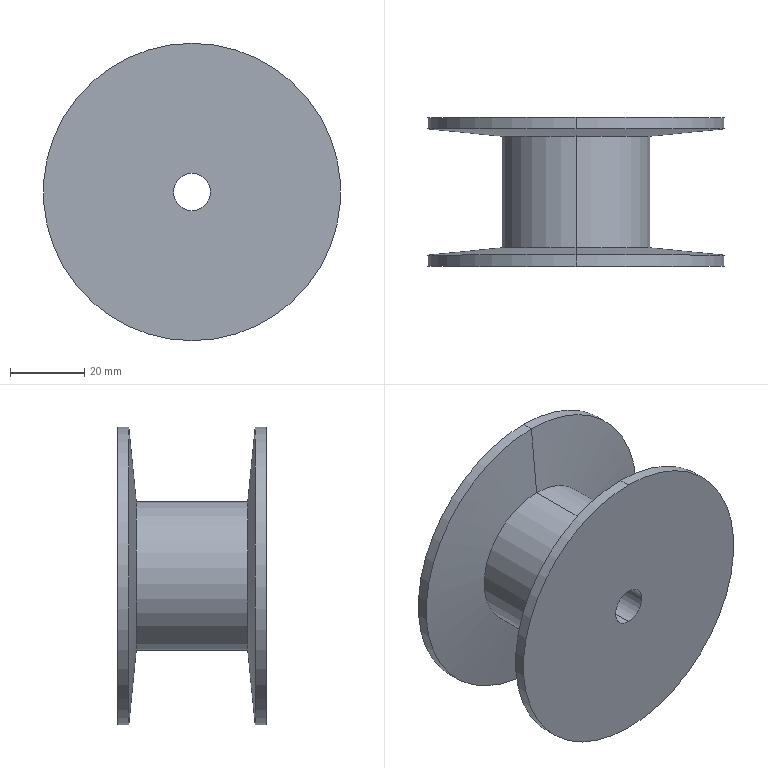Part | SolidWorks | features Revolution 1 | 1 solid | 14 faces | box 80 x 40 x 80 mm | volume 76445 mm3 | cylinder 8 | cone 4 | plane 2 | commonest cylinder face diameters 80 x4 10 x2 40 x2
STEP:
#1=CARTESIAN_POINT('',(0.,40.,5.));
#2=VERTEX_POINT('',#1);
#3=CARTESIAN_POINT('',(0.,40.,-5.));
#4=VERTEX_POINT('',#3);
#5=CARTESIAN_POINT('',(0.,40.,0.));
#6=DIRECTION('',(0.,-1.,0.));
#7=DIRECTION('',(0.,0.,-1.));
#8=AXIS2_PLACEMENT_3D('',#5,#6,#7);
#9=CIRCLE('',#8,5.);
#10=EDGE_CURVE('',#2,#4,#9,.T.);
#11=ORIENTED_EDGE('',*,*,#10,.F.);
#12=CARTESIAN_POINT('',(0.,0.,5.));
#13=VERTEX_POINT('',#12);
#14=CARTESIAN_POINT('',(0.,0.,5.));
#15=DIRECTION('',(0.,-1.,0.));
#16=VECTOR('',#15,1000.);
#17=LINE('',#14,#16);
#18=EDGE_CURVE('',#2,#13,#17,.T.);
#19=ORIENTED_EDGE('',*,*,#18,.T.);
#20=CARTESIAN_POINT('',(0.,0.,-5.));
#21=VERTEX_POINT('',#20);
#22=CARTESIAN_POINT('',(0.,0.,0.));
#23=DIRECTION('',(0.,-1.,0.));
#24=DIRECTION('',(0.,0.,-1.));
#25=AXIS2_PLACEMENT_3D('',#22,#23,#24);
#26=CIRCLE('',#25,5.);
#27=EDGE_CURVE('',#13,#21,#26,.T.);
#28=ORIENTED_EDGE('',*,*,#27,.T.);
#29=CARTESIAN_POINT('',(0.,0.,-5.));
#30=DIRECTION('',(0.,-1.,0.));
#31=VECTOR('',#30,1000.);
#32=LINE('',#29,#31);
#33=EDGE_CURVE('',#4,#21,#32,.T.);
#34=ORIENTED_EDGE('',*,*,#33,.F.);
#35=EDGE_LOOP('',(#11,#19,#28,#34));
#36=FACE_OUTER_BOUND('',#35,.T.);
#37=CARTESIAN_POINT('',(0.,0.,0.));
#38=DIRECTION('',(0.,-1.,0.));
#39=DIRECTION('',(0.,0.,-1.));
#40=AXIS2_PLACEMENT_3D('',#37,#38,#39);
#41=CYLINDRICAL_SURFACE('',#40,5.);
#42=ADVANCED_FACE('',(#36),#41,.F.);
#43=CARTESIAN_POINT('',(0.,40.,-40.));
#44=VERTEX_POINT('',#43);
#45=CARTESIAN_POINT('',(0.,40.,40.));
#46=VERTEX_POINT('',#45);
#47=CARTESIAN_POINT('',(0.,40.,0.));
#48=DIRECTION('',(0.,-1.,0.));
#49=DIRECTION('',(0.,0.,-1.));
#50=AXIS2_PLACEMENT_3D('',#47,#48,#49);
#51=CIRCLE('',#50,40.);
#52=EDGE_CURVE('',#44,#46,#51,.T.);
#53=ORIENTED_EDGE('',*,*,#52,.T.);
#54=CARTESIAN_POINT('',(0.,37.,40.));
#55=VERTEX_POINT('',#54);
#56=CARTESIAN_POINT('',(0.,0.,40.));
#57=DIRECTION('',(0.,-1.,0.));
#58=VECTOR('',#57,1000.);
#59=LINE('',#56,#58);
#60=EDGE_CURVE('',#46,#55,#59,.T.);
#61=ORIENTED_EDGE('',*,*,#60,.T.);
#62=CARTESIAN_POINT('',(0.,37.,-40.));
#63=VERTEX_POINT('',#62);
#64=CARTESIAN_POINT('',(0.,37.,0.));
#65=DIRECTION('',(0.,-1.,0.));
#66=DIRECTION('',(0.,0.,-1.));
#67=AXIS2_PLACEMENT_3D('',#64,#65,#66);
#68=CIRCLE('',#67,40.);
#69=EDGE_CURVE('',#63,#55,#68,.T.);
#70=ORIENTED_EDGE('',*,*,#69,.F.);
#71=CARTESIAN_POINT('',(0.,0.,-40.));
#72=DIRECTION('',(0.,-1.,0.));
#73=VECTOR('',#72,1000.);
#74=LINE('',#71,#73);
#75=EDGE_CURVE('',#44,#63,#74,.T.);
#76=ORIENTED_EDGE('',*,*,#75,.F.);
#77=EDGE_LOOP('',(#53,#61,#70,#76));
#78=FACE_OUTER_BOUND('',#77,.T.);
#79=CARTESIAN_POINT('',(0.,0.,0.));
#80=DIRECTION('',(0.,-1.,0.));
#81=DIRECTION('',(0.,0.,-1.));
#82=AXIS2_PLACEMENT_3D('',#79,#80,#81);
#83=CYLINDRICAL_SURFACE('',#82,40.);
#84=ADVANCED_FACE('',(#78),#83,.T.);
#85=CARTESIAN_POINT('',(0.,35.,-20.));
#86=VERTEX_POINT('',#85);
#87=CARTESIAN_POINT('',(0.,35.,20.));
#88=VERTEX_POINT('',#87);
#89=CARTESIAN_POINT('',(0.,35.,0.));
#90=DIRECTION('',(0.,-1.,0.));
#91=DIRECTION('',(0.,0.,-1.));
#92=AXIS2_PLACEMENT_3D('',#89,#90,#91);
#93=CIRCLE('',#92,20.);
#94=EDGE_CURVE('',#86,#88,#93,.T.);
#95=ORIENTED_EDGE('',*,*,#94,.F.);
#96=CARTESIAN_POINT('',(0.,35.,-20.));
#97=DIRECTION('',(0.,0.0995,-0.995));
#98=VECTOR('',#97,1000.);
#99=LINE('',#96,#98);
#100=EDGE_CURVE('',#86,#63,#99,.T.);
#101=ORIENTED_EDGE('',*,*,#100,.T.);
#102=ORIENTED_EDGE('',*,*,#69,.T.);
#103=CARTESIAN_POINT('',(0.,35.,20.));
#104=DIRECTION('',(0.,0.0995,0.995));
#105=VECTOR('',#104,1000.);
#106=LINE('',#103,#105);
#107=EDGE_CURVE('',#88,#55,#106,.T.);
#108=ORIENTED_EDGE('',*,*,#107,.F.);
#109=EDGE_LOOP('',(#95,#101,#102,#108));
#110=FACE_OUTER_BOUND('',#109,.T.);
#111=CARTESIAN_POINT('',(0.,35.,0.));
#112=DIRECTION('',(0.,1.,0.));
#113=DIRECTION('',(0.,0.,1.));
#114=AXIS2_PLACEMENT_3D('',#111,#112,#113);
#115=CONICAL_SURFACE('',#114,20.,1.471);
#116=ADVANCED_FACE('',(#110),#115,.T.);
#117=ORIENTED_EDGE('',*,*,#94,.T.);
#118=CARTESIAN_POINT('',(0.,5.,20.));
#119=VERTEX_POINT('',#118);
#120=CARTESIAN_POINT('',(0.,0.,20.));
#121=DIRECTION('',(0.,-1.,0.));
#122=VECTOR('',#121,1000.);
#123=LINE('',#120,#122);
#124=EDGE_CURVE('',#88,#119,#123,.T.);
#125=ORIENTED_EDGE('',*,*,#124,.T.);
#126=CARTESIAN_POINT('',(0.,5.,-20.));
#127=VERTEX_POINT('',#126);
#128=CARTESIAN_POINT('',(0.,5.,0.));
#129=DIRECTION('',(0.,-1.,0.));
#130=DIRECTION('',(0.,0.,-1.));
#131=AXIS2_PLACEMENT_3D('',#128,#129,#130);
#132=CIRCLE('',#131,20.);
#133=EDGE_CURVE('',#127,#119,#132,.T.);
#134=ORIENTED_EDGE('',*,*,#133,.F.);
#135=CARTESIAN_POINT('',(0.,0.,-20.));
#136=DIRECTION('',(0.,-1.,0.));
#137=VECTOR('',#136,1000.);
#138=LINE('',#135,#137);
#139=EDGE_CURVE('',#86,#127,#138,.T.);
#140=ORIENTED_EDGE('',*,*,#139,.F.);
#141=EDGE_LOOP('',(#117,#125,#134,#140));
#142=FACE_OUTER_BOUND('',#141,.T.);
#143=CARTESIAN_POINT('',(0.,0.,0.));
#144=DIRECTION('',(0.,-1.,0.));
#145=DIRECTION('',(0.,0.,-1.));
#146=AXIS2_PLACEMENT_3D('',#143,#144,#145);
#147=CYLINDRICAL_SURFACE('',#146,20.);
#148=ADVANCED_FACE('',(#142),#147,.T.);
#149=ORIENTED_EDGE('',*,*,#133,.T.);
#150=CARTESIAN_POINT('',(0.,3.,40.));
#151=VERTEX_POINT('',#150);
#152=CARTESIAN_POINT('',(0.,3.,40.));
#153=DIRECTION('',(0.,-0.0995,0.995));
#154=VECTOR('',#153,1000.);
#155=LINE('',#152,#154);
#156=EDGE_CURVE('',#119,#151,#155,.T.);
#157=ORIENTED_EDGE('',*,*,#156,.T.);
#158=CARTESIAN_POINT('',(0.,3.,-40.));
#159=VERTEX_POINT('',#158);
#160=CARTESIAN_POINT('',(0.,3.,0.));
#161=DIRECTION('',(0.,-1.,0.));
#162=DIRECTION('',(0.,0.,-1.));
#163=AXIS2_PLACEMENT_3D('',#160,#161,#162);
#164=CIRCLE('',#163,40.);
#165=EDGE_CURVE('',#159,#151,#164,.T.);
#166=ORIENTED_EDGE('',*,*,#165,.F.);
#167=CARTESIAN_POINT('',(0.,3.,-40.));
#168=DIRECTION('',(0.,-0.0995,-0.995));
#169=VECTOR('',#168,1000.);
#170=LINE('',#167,#169);
#171=EDGE_CURVE('',#127,#159,#170,.T.);
#172=ORIENTED_EDGE('',*,*,#171,.F.);
#173=EDGE_LOOP('',(#149,#157,#166,#172));
#174=FACE_OUTER_BOUND('',#173,.T.);
#175=CARTESIAN_POINT('',(0.,3.,0.));
#176=DIRECTION('',(0.,-1.,0.));
#177=DIRECTION('',(0.,0.,-1.));
#178=AXIS2_PLACEMENT_3D('',#175,#176,#177);
#179=CONICAL_SURFACE('',#178,40.,1.471);
#180=ADVANCED_FACE('',(#174),#179,.T.);
#181=ORIENTED_EDGE('',*,*,#165,.T.);
#182=CARTESIAN_POINT('',(0.,0.,40.));
#183=VERTEX_POINT('',#182);
#184=CARTESIAN_POINT('',(0.,0.,40.));
#185=DIRECTION('',(0.,-1.,0.));
#186=VECTOR('',#185,1000.);
#187=LINE('',#184,#186);
#188=EDGE_CURVE('',#151,#183,#187,.T.);
#189=ORIENTED_EDGE('',*,*,#188,.T.);
#190=CARTESIAN_POINT('',(0.,0.,-40.));
#191=VERTEX_POINT('',#190);
#192=CARTESIAN_POINT('',(0.,0.,0.));
#193=DIRECTION('',(0.,-1.,0.));
#194=DIRECTION('',(0.,0.,-1.));
#195=AXIS2_PLACEMENT_3D('',#192,#193,#194);
#196=CIRCLE('',#195,40.);
#197=EDGE_CURVE('',#191,#183,#196,.T.);
#198=ORIENTED_EDGE('',*,*,#197,.F.);
#199=CARTESIAN_POINT('',(0.,0.,-40.));
#200=DIRECTION('',(0.,-1.,0.));
#201=VECTOR('',#200,1000.);
#202=LINE('',#199,#201);
#203=EDGE_CURVE('',#159,#191,#202,.T.);
#204=ORIENTED_EDGE('',*,*,#203,.F.);
#205=EDGE_LOOP('',(#181,#189,#198,#204));
#206=FACE_OUTER_BOUND('',#205,.T.);
#207=CARTESIAN_POINT('',(0.,0.,0.));
#208=DIRECTION('',(0.,-1.,0.));
#209=DIRECTION('',(0.,0.,-1.));
#210=AXIS2_PLACEMENT_3D('',#207,#208,#209);
#211=CYLINDRICAL_SURFACE('',#210,40.);
#212=ADVANCED_FACE('',(#206),#211,.T.);
#213=ORIENTED_EDGE('',*,*,#188,.F.);
#214=CARTESIAN_POINT('',(0.,3.,0.));
#215=DIRECTION('',(0.,-1.,0.));
#216=DIRECTION('',(0.,0.,-1.));
#217=AXIS2_PLACEMENT_3D('',#214,#215,#216);
#218=CIRCLE('',#217,40.);
#219=EDGE_CURVE('',#151,#159,#218,.T.);
#220=ORIENTED_EDGE('',*,*,#219,.T.);
#221=ORIENTED_EDGE('',*,*,#203,.T.);
#222=CARTESIAN_POINT('',(0.,0.,0.));
#223=DIRECTION('',(0.,-1.,0.));
#224=DIRECTION('',(0.,0.,-1.));
#225=AXIS2_PLACEMENT_3D('',#222,#223,#224);
#226=CIRCLE('',#225,40.);
#227=EDGE_CURVE('',#183,#191,#226,.T.);
#228=ORIENTED_EDGE('',*,*,#227,.F.);
#229=EDGE_LOOP('',(#213,#220,#221,#228));
#230=FACE_OUTER_BOUND('',#229,.T.);
#231=CARTESIAN_POINT('',(0.,0.,0.));
#232=DIRECTION('',(0.,-1.,0.));
#233=DIRECTION('',(0.,0.,-1.));
#234=AXIS2_PLACEMENT_3D('',#231,#232,#233);
#235=CYLINDRICAL_SURFACE('',#234,40.);
#236=ADVANCED_FACE('',(#230),#235,.T.);
#237=ORIENTED_EDGE('',*,*,#156,.F.);
#238=CARTESIAN_POINT('',(0.,5.,0.));
#239=DIRECTION('',(0.,-1.,0.));
#240=DIRECTION('',(0.,0.,-1.));
#241=AXIS2_PLACEMENT_3D('',#238,#239,#240);
#242=CIRCLE('',#241,20.);
#243=EDGE_CURVE('',#119,#127,#242,.T.);
#244=ORIENTED_EDGE('',*,*,#243,.T.);
#245=ORIENTED_EDGE('',*,*,#171,.T.);
#246=ORIENTED_EDGE('',*,*,#219,.F.);
#247=EDGE_LOOP('',(#237,#244,#245,#246));
#248=FACE_OUTER_BOUND('',#247,.T.);
#249=CARTESIAN_POINT('',(0.,3.,0.));
#250=DIRECTION('',(0.,-1.,0.));
#251=DIRECTION('',(0.,0.,-1.));
#252=AXIS2_PLACEMENT_3D('',#249,#250,#251);
#253=CONICAL_SURFACE('',#252,40.,1.471);
#254=ADVANCED_FACE('',(#248),#253,.T.);
#255=ORIENTED_EDGE('',*,*,#124,.F.);
#256=CARTESIAN_POINT('',(0.,35.,0.));
#257=DIRECTION('',(0.,-1.,0.));
#258=DIRECTION('',(0.,0.,-1.));
#259=AXIS2_PLACEMENT_3D('',#256,#257,#258);
#260=CIRCLE('',#259,20.);
#261=EDGE_CURVE('',#88,#86,#260,.T.);
#262=ORIENTED_EDGE('',*,*,#261,.T.);
#263=ORIENTED_EDGE('',*,*,#139,.T.);
#264=ORIENTED_EDGE('',*,*,#243,.F.);
#265=EDGE_LOOP('',(#255,#262,#263,#264));
#266=FACE_OUTER_BOUND('',#265,.T.);
#267=CARTESIAN_POINT('',(0.,0.,0.));
#268=DIRECTION('',(0.,-1.,0.));
#269=DIRECTION('',(0.,0.,-1.));
#270=AXIS2_PLACEMENT_3D('',#267,#268,#269);
#271=CYLINDRICAL_SURFACE('',#270,20.);
#272=ADVANCED_FACE('',(#266),#271,.T.);
#273=ORIENTED_EDGE('',*,*,#100,.F.);
#274=ORIENTED_EDGE('',*,*,#261,.F.);
#275=ORIENTED_EDGE('',*,*,#107,.T.);
#276=CARTESIAN_POINT('',(0.,37.,0.));
#277=DIRECTION('',(0.,-1.,0.));
#278=DIRECTION('',(0.,0.,-1.));
#279=AXIS2_PLACEMENT_3D('',#276,#277,#278);
#280=CIRCLE('',#279,40.);
#281=EDGE_CURVE('',#55,#63,#280,.T.);
#282=ORIENTED_EDGE('',*,*,#281,.T.);
#283=EDGE_LOOP('',(#273,#274,#275,#282));
#284=FACE_OUTER_BOUND('',#283,.T.);
#285=CARTESIAN_POINT('',(0.,35.,0.));
#286=DIRECTION('',(0.,1.,0.));
#287=DIRECTION('',(0.,0.,1.));
#288=AXIS2_PLACEMENT_3D('',#285,#286,#287);
#289=CONICAL_SURFACE('',#288,20.,1.471);
#290=ADVANCED_FACE('',(#284),#289,.T.);
#291=ORIENTED_EDGE('',*,*,#60,.F.);
#292=CARTESIAN_POINT('',(0.,40.,0.));
#293=DIRECTION('',(0.,-1.,0.));
#294=DIRECTION('',(0.,0.,-1.));
#295=AXIS2_PLACEMENT_3D('',#292,#293,#294);
#296=CIRCLE('',#295,40.);
#297=EDGE_CURVE('',#46,#44,#296,.T.);
#298=ORIENTED_EDGE('',*,*,#297,.T.);
#299=ORIENTED_EDGE('',*,*,#75,.T.);
#300=ORIENTED_EDGE('',*,*,#281,.F.);
#301=EDGE_LOOP('',(#291,#298,#299,#300));
#302=FACE_OUTER_BOUND('',#301,.T.);
#303=CARTESIAN_POINT('',(0.,0.,0.));
#304=DIRECTION('',(0.,-1.,0.));
#305=DIRECTION('',(0.,0.,-1.));
#306=AXIS2_PLACEMENT_3D('',#303,#304,#305);
#307=CYLINDRICAL_SURFACE('',#306,40.);
#308=ADVANCED_FACE('',(#302),#307,.T.);
#309=CARTESIAN_POINT('',(0.,40.,0.));
#310=DIRECTION('',(0.,-1.,0.));
#311=DIRECTION('',(0.,0.,-1.));
#312=AXIS2_PLACEMENT_3D('',#309,#310,#311);
#313=CIRCLE('',#312,5.);
#314=EDGE_CURVE('',#4,#2,#313,.T.);
#315=ORIENTED_EDGE('',*,*,#314,.T.);
#316=ORIENTED_EDGE('',*,*,#10,.T.);
#317=EDGE_LOOP('',(#315,#316));
#318=FACE_BOUND('',#317,.T.);
#319=ORIENTED_EDGE('',*,*,#52,.F.);
#320=ORIENTED_EDGE('',*,*,#297,.F.);
#321=EDGE_LOOP('',(#319,#320));
#322=FACE_OUTER_BOUND('',#321,.T.);
#323=CARTESIAN_POINT('',(0.,40.,-40.));
#324=DIRECTION('',(0.,1.,0.));
#325=DIRECTION('',(0.,0.,1.));
#326=AXIS2_PLACEMENT_3D('',#323,#324,#325);
#327=PLANE('',#326);
#328=ADVANCED_FACE('',(#318,#322),#327,.T.);
#329=ORIENTED_EDGE('',*,*,#18,.F.);
#330=ORIENTED_EDGE('',*,*,#314,.F.);
#331=ORIENTED_EDGE('',*,*,#33,.T.);
#332=CARTESIAN_POINT('',(0.,0.,0.));
#333=DIRECTION('',(0.,-1.,0.));
#334=DIRECTION('',(0.,0.,-1.));
#335=AXIS2_PLACEMENT_3D('',#332,#333,#334);
#336=CIRCLE('',#335,5.);
#337=EDGE_CURVE('',#21,#13,#336,.T.);
#338=ORIENTED_EDGE('',*,*,#337,.T.);
#339=EDGE_LOOP('',(#329,#330,#331,#338));
#340=FACE_OUTER_BOUND('',#339,.T.);
#341=CARTESIAN_POINT('',(0.,0.,0.));
#342=DIRECTION('',(0.,-1.,0.));
#343=DIRECTION('',(0.,0.,-1.));
#344=AXIS2_PLACEMENT_3D('',#341,#342,#343);
#345=CYLINDRICAL_SURFACE('',#344,5.);
#346=ADVANCED_FACE('',(#340),#345,.F.);
#347=ORIENTED_EDGE('',*,*,#197,.T.);
#348=ORIENTED_EDGE('',*,*,#227,.T.);
#349=EDGE_LOOP('',(#347,#348));
#350=FACE_OUTER_BOUND('',#349,.T.);
#351=ORIENTED_EDGE('',*,*,#337,.F.);
#352=ORIENTED_EDGE('',*,*,#27,.F.);
#353=EDGE_LOOP('',(#351,#352));
#354=FACE_BOUND('',#353,.T.);
#355=CARTESIAN_POINT('',(0.,0.,-5.));
#356=DIRECTION('',(0.,-1.,0.));
#357=DIRECTION('',(0.,0.,-1.));
#358=AXIS2_PLACEMENT_3D('',#355,#356,#357);
#359=PLANE('',#358);
#360=ADVANCED_FACE('',(#350,#354),#359,.T.);
#361=CLOSED_SHELL('',(#42,#84,#116,#148,#180,#212,#236,#254,#272,#290,#308,#328,#346,#360));
#362=MANIFOLD_SOLID_BREP('',#361);
#363=CARTESIAN_POINT('',(0.,0.,0.));
#364=DIRECTION('',(0.,0.,1.));
#365=DIRECTION('',(1.,0.,0.));
#366=AXIS2_PLACEMENT_3D('',#363,#364,#365);
#367=(LENGTH_UNIT()NAMED_UNIT(*)SI_UNIT(.MILLI.,.METRE.));
#368=UNCERTAINTY_MEASURE_WITH_UNIT(LENGTH_MEASURE(0.00001),#367,'','');
#369=(NAMED_UNIT(*)PLANE_ANGLE_UNIT()SI_UNIT($,.RADIAN.));
#370=(NAMED_UNIT(*)SI_UNIT($,.STERADIAN.)SOLID_ANGLE_UNIT());
#371=(GEOMETRIC_REPRESENTATION_CONTEXT(3)GLOBAL_UNCERTAINTY_ASSIGNED_CONTEXT((#368))GLOBAL_UNIT_ASSIGNED_CONTEXT((#367,#369,#370))REPRESENTATION_CONTEXT('',''));
#372=ADVANCED_BREP_SHAPE_REPRESENTATION('',(#362,#366),#371);